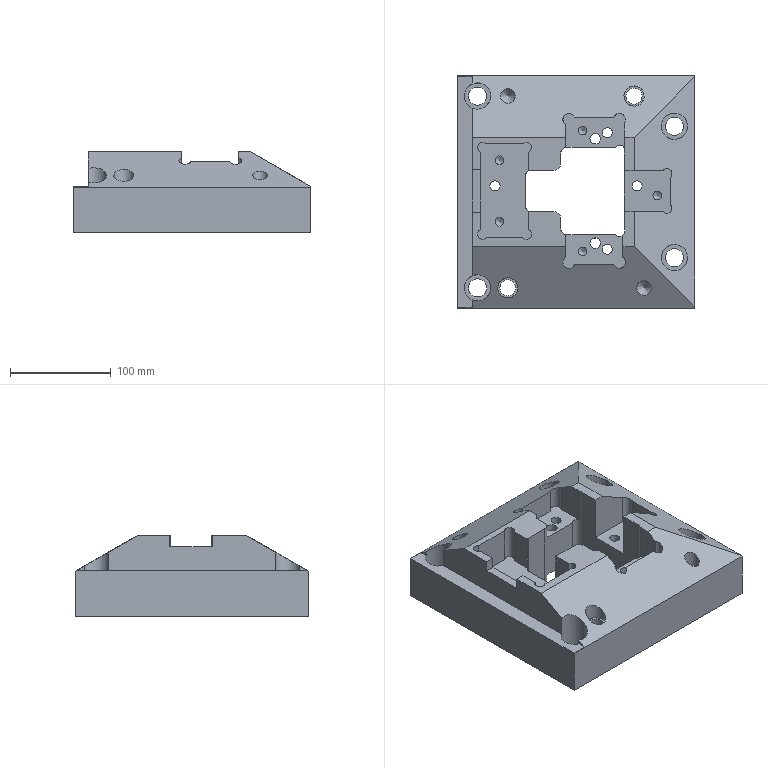Part | STEP file | 180_id4502_x_t | 1 solid | 101 faces | box 235 x 230 x 80 mm | volume 2542104 mm3 | plane 51 | cylinder 43 | cone 7 | commonest cylinder face diameters 10 x14 12 x6 8.506 x5 18.009 x4 26.008 x4 10.5 x2